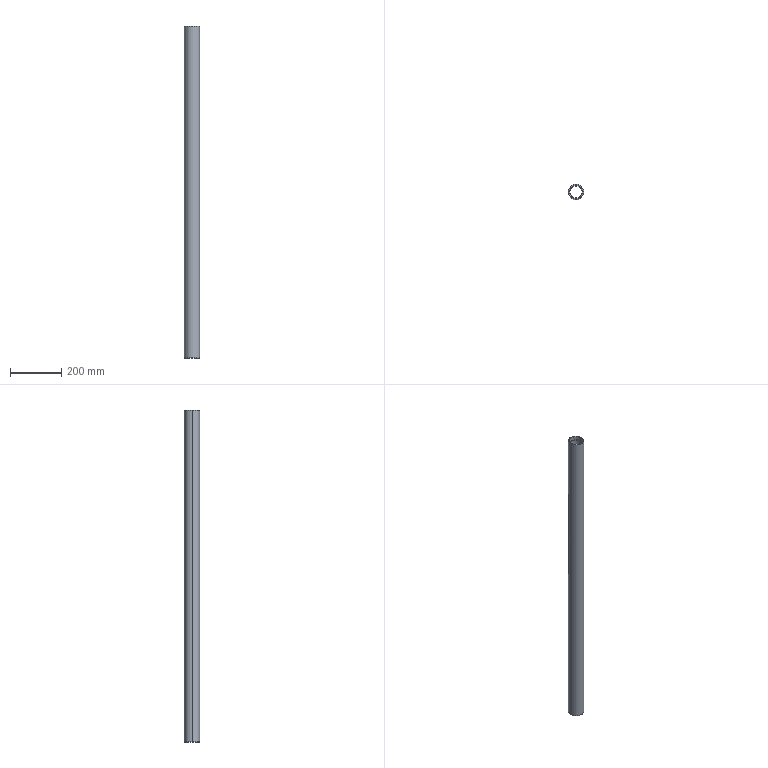Part | SolidWorks | features ICE 3, Chamfer 1, Extrusion 1 | 1 solid | 20 faces | box 60 x 60 x 1300 mm | volume 1313726 mm3 | cone 8 | cylinder 8 | plane 4 | commonest cylinder face diameters 52 x4 48 x2 60 x2
STEP:
#1=CARTESIAN_POINT('',(29.5,0.,1300.));
#2=VERTEX_POINT('',#1);
#3=CARTESIAN_POINT('',(-29.5,0.,1300.));
#4=VERTEX_POINT('',#3);
#5=CARTESIAN_POINT('',(0.,0.,1300.));
#6=DIRECTION('',(0.,0.,1.));
#7=DIRECTION('',(1.,0.,0.));
#8=AXIS2_PLACEMENT_3D('',#5,#6,#7);
#9=CIRCLE('',#8,29.5);
#10=EDGE_CURVE('',#2,#4,#9,.T.);
#11=ORIENTED_EDGE('',*,*,#10,.F.);
#12=CARTESIAN_POINT('',(30.,0.,1299.5));
#13=VERTEX_POINT('',#12);
#14=CARTESIAN_POINT('',(29.5,0.,1300.));
#15=DIRECTION('',(0.7071,0.,-0.7071));
#16=VECTOR('',#15,1000.);
#17=LINE('',#14,#16);
#18=EDGE_CURVE('',#2,#13,#17,.T.);
#19=ORIENTED_EDGE('',*,*,#18,.T.);
#20=CARTESIAN_POINT('',(-30.,0.,1299.5));
#21=VERTEX_POINT('',#20);
#22=CARTESIAN_POINT('',(0.,0.,1299.5));
#23=DIRECTION('',(0.,0.,-1.));
#24=DIRECTION('',(1.,0.,0.));
#25=AXIS2_PLACEMENT_3D('',#22,#23,#24);
#26=CIRCLE('',#25,30.);
#27=EDGE_CURVE('',#21,#13,#26,.T.);
#28=ORIENTED_EDGE('',*,*,#27,.F.);
#29=CARTESIAN_POINT('',(-29.5,0.,1300.));
#30=DIRECTION('',(-0.7071,0.,-0.7071));
#31=VECTOR('',#30,1000.);
#32=LINE('',#29,#31);
#33=EDGE_CURVE('',#4,#21,#32,.T.);
#34=ORIENTED_EDGE('',*,*,#33,.F.);
#35=EDGE_LOOP('',(#11,#19,#28,#34));
#36=FACE_OUTER_BOUND('',#35,.T.);
#37=CARTESIAN_POINT('',(0.,0.,1300.));
#38=DIRECTION('',(0.,0.,-1.));
#39=DIRECTION('',(-1.,0.,0.));
#40=AXIS2_PLACEMENT_3D('',#37,#38,#39);
#41=CONICAL_SURFACE('',#40,29.5,0.7854);
#42=ADVANCED_FACE('',(#36),#41,.T.);
#43=CARTESIAN_POINT('',(-26.,0.,1299.5));
#44=VERTEX_POINT('',#43);
#45=CARTESIAN_POINT('',(26.,0.,1299.5));
#46=VERTEX_POINT('',#45);
#47=CARTESIAN_POINT('',(0.,0.,1299.5));
#48=DIRECTION('',(0.,0.,1.));
#49=DIRECTION('',(1.,0.,0.));
#50=AXIS2_PLACEMENT_3D('',#47,#48,#49);
#51=CIRCLE('',#50,26.);
#52=EDGE_CURVE('',#44,#46,#51,.T.);
#53=ORIENTED_EDGE('',*,*,#52,.F.);
#54=CARTESIAN_POINT('',(-26.5,0.,1300.));
#55=VERTEX_POINT('',#54);
#56=CARTESIAN_POINT('',(-26.,0.,1299.5));
#57=DIRECTION('',(-0.7071,0.,0.7071));
#58=VECTOR('',#57,1000.);
#59=LINE('',#56,#58);
#60=EDGE_CURVE('',#44,#55,#59,.T.);
#61=ORIENTED_EDGE('',*,*,#60,.T.);
#62=CARTESIAN_POINT('',(26.5,0.,1300.));
#63=VERTEX_POINT('',#62);
#64=CARTESIAN_POINT('',(0.,0.,1300.));
#65=DIRECTION('',(0.,0.,-1.));
#66=DIRECTION('',(1.,0.,0.));
#67=AXIS2_PLACEMENT_3D('',#64,#65,#66);
#68=CIRCLE('',#67,26.5);
#69=EDGE_CURVE('',#63,#55,#68,.T.);
#70=ORIENTED_EDGE('',*,*,#69,.F.);
#71=CARTESIAN_POINT('',(26.,0.,1299.5));
#72=DIRECTION('',(0.7071,0.,0.7071));
#73=VECTOR('',#72,1000.);
#74=LINE('',#71,#73);
#75=EDGE_CURVE('',#46,#63,#74,.T.);
#76=ORIENTED_EDGE('',*,*,#75,.F.);
#77=EDGE_LOOP('',(#53,#61,#70,#76));
#78=FACE_OUTER_BOUND('',#77,.T.);
#79=CARTESIAN_POINT('',(0.,0.,1299.5));
#80=DIRECTION('',(0.,0.,1.));
#81=DIRECTION('',(1.,0.,0.));
#82=AXIS2_PLACEMENT_3D('',#79,#80,#81);
#83=CONICAL_SURFACE('',#82,26.,0.7854);
#84=ADVANCED_FACE('',(#78),#83,.F.);
#85=CARTESIAN_POINT('',(-29.5,0.,0.));
#86=VERTEX_POINT('',#85);
#87=CARTESIAN_POINT('',(29.5,0.,0.));
#88=VERTEX_POINT('',#87);
#89=CARTESIAN_POINT('',(0.,0.,0.));
#90=DIRECTION('',(0.,0.,-1.));
#91=DIRECTION('',(1.,0.,0.));
#92=AXIS2_PLACEMENT_3D('',#89,#90,#91);
#93=CIRCLE('',#92,29.5);
#94=EDGE_CURVE('',#86,#88,#93,.T.);
#95=ORIENTED_EDGE('',*,*,#94,.F.);
#96=CARTESIAN_POINT('',(-30.,0.,0.5));
#97=VERTEX_POINT('',#96);
#98=CARTESIAN_POINT('',(-30.,0.,0.5));
#99=DIRECTION('',(-0.7071,0.,0.7071));
#100=VECTOR('',#99,1000.);
#101=LINE('',#98,#100);
#102=EDGE_CURVE('',#86,#97,#101,.T.);
#103=ORIENTED_EDGE('',*,*,#102,.T.);
#104=CARTESIAN_POINT('',(30.,0.,0.5));
#105=VERTEX_POINT('',#104);
#106=CARTESIAN_POINT('',(0.,0.,0.5));
#107=DIRECTION('',(0.,0.,1.));
#108=DIRECTION('',(1.,0.,0.));
#109=AXIS2_PLACEMENT_3D('',#106,#107,#108);
#110=CIRCLE('',#109,30.);
#111=EDGE_CURVE('',#105,#97,#110,.T.);
#112=ORIENTED_EDGE('',*,*,#111,.F.);
#113=CARTESIAN_POINT('',(30.,0.,0.5));
#114=DIRECTION('',(0.7071,0.,0.7071));
#115=VECTOR('',#114,1000.);
#116=LINE('',#113,#115);
#117=EDGE_CURVE('',#88,#105,#116,.T.);
#118=ORIENTED_EDGE('',*,*,#117,.F.);
#119=EDGE_LOOP('',(#95,#103,#112,#118));
#120=FACE_OUTER_BOUND('',#119,.T.);
#121=CARTESIAN_POINT('',(0.,0.,0.5));
#122=DIRECTION('',(0.,0.,1.));
#123=DIRECTION('',(1.,0.,0.));
#124=AXIS2_PLACEMENT_3D('',#121,#122,#123);
#125=CONICAL_SURFACE('',#124,30.,0.7854);
#126=ADVANCED_FACE('',(#120),#125,.T.);
#127=CARTESIAN_POINT('',(26.,0.,0.5));
#128=VERTEX_POINT('',#127);
#129=CARTESIAN_POINT('',(-26.,0.,0.5));
#130=VERTEX_POINT('',#129);
#131=CARTESIAN_POINT('',(0.,0.,0.5));
#132=DIRECTION('',(0.,0.,-1.));
#133=DIRECTION('',(1.,0.,0.));
#134=AXIS2_PLACEMENT_3D('',#131,#132,#133);
#135=CIRCLE('',#134,26.);
#136=EDGE_CURVE('',#128,#130,#135,.T.);
#137=ORIENTED_EDGE('',*,*,#136,.F.);
#138=CARTESIAN_POINT('',(26.5,0.,0.));
#139=VERTEX_POINT('',#138);
#140=CARTESIAN_POINT('',(26.,0.,0.5));
#141=DIRECTION('',(0.7071,0.,-0.7071));
#142=VECTOR('',#141,1000.);
#143=LINE('',#140,#142);
#144=EDGE_CURVE('',#128,#139,#143,.T.);
#145=ORIENTED_EDGE('',*,*,#144,.T.);
#146=CARTESIAN_POINT('',(-26.5,0.,0.));
#147=VERTEX_POINT('',#146);
#148=CARTESIAN_POINT('',(0.,0.,0.));
#149=DIRECTION('',(0.,0.,1.));
#150=DIRECTION('',(1.,0.,0.));
#151=AXIS2_PLACEMENT_3D('',#148,#149,#150);
#152=CIRCLE('',#151,26.5);
#153=EDGE_CURVE('',#147,#139,#152,.T.);
#154=ORIENTED_EDGE('',*,*,#153,.F.);
#155=CARTESIAN_POINT('',(-26.,0.,0.5));
#156=DIRECTION('',(-0.7071,0.,-0.7071));
#157=VECTOR('',#156,1000.);
#158=LINE('',#155,#157);
#159=EDGE_CURVE('',#130,#147,#158,.T.);
#160=ORIENTED_EDGE('',*,*,#159,.F.);
#161=EDGE_LOOP('',(#137,#145,#154,#160));
#162=FACE_OUTER_BOUND('',#161,.T.);
#163=CARTESIAN_POINT('',(0.,0.,0.5));
#164=DIRECTION('',(0.,0.,-1.));
#165=DIRECTION('',(-1.,0.,0.));
#166=AXIS2_PLACEMENT_3D('',#163,#164,#165);
#167=CONICAL_SURFACE('',#166,26.,0.7854);
#168=ADVANCED_FACE('',(#162),#167,.F.);
#169=CARTESIAN_POINT('',(-26.,0.,1285.));
#170=VERTEX_POINT('',#169);
#171=CARTESIAN_POINT('',(26.,0.,1285.));
#172=VERTEX_POINT('',#171);
#173=CARTESIAN_POINT('',(0.,0.,1285.));
#174=DIRECTION('',(0.,0.,1.));
#175=DIRECTION('',(1.,0.,0.));
#176=AXIS2_PLACEMENT_3D('',#173,#174,#175);
#177=CIRCLE('',#176,26.);
#178=EDGE_CURVE('',#170,#172,#177,.T.);
#179=ORIENTED_EDGE('',*,*,#178,.F.);
#180=CARTESIAN_POINT('',(-26.,0.,1285.));
#181=DIRECTION('',(0.,0.,1.));
#182=VECTOR('',#181,1000.);
#183=LINE('',#180,#182);
#184=EDGE_CURVE('',#170,#44,#183,.T.);
#185=ORIENTED_EDGE('',*,*,#184,.T.);
#186=ORIENTED_EDGE('',*,*,#52,.T.);
#187=CARTESIAN_POINT('',(26.,0.,1285.));
#188=DIRECTION('',(0.,0.,1.));
#189=VECTOR('',#188,1000.);
#190=LINE('',#187,#189);
#191=EDGE_CURVE('',#172,#46,#190,.T.);
#192=ORIENTED_EDGE('',*,*,#191,.F.);
#193=EDGE_LOOP('',(#179,#185,#186,#192));
#194=FACE_OUTER_BOUND('',#193,.T.);
#195=CARTESIAN_POINT('',(0.,0.,1285.));
#196=DIRECTION('',(0.,0.,1.));
#197=DIRECTION('',(1.,0.,0.));
#198=AXIS2_PLACEMENT_3D('',#195,#196,#197);
#199=CYLINDRICAL_SURFACE('',#198,26.);
#200=ADVANCED_FACE('',(#194),#199,.F.);
#201=CARTESIAN_POINT('',(26.,0.,15.));
#202=VERTEX_POINT('',#201);
#203=CARTESIAN_POINT('',(-26.,0.,15.));
#204=VERTEX_POINT('',#203);
#205=CARTESIAN_POINT('',(0.,0.,15.));
#206=DIRECTION('',(0.,0.,-1.));
#207=DIRECTION('',(-1.,0.,0.));
#208=AXIS2_PLACEMENT_3D('',#205,#206,#207);
#209=CIRCLE('',#208,26.);
#210=EDGE_CURVE('',#202,#204,#209,.T.);
#211=ORIENTED_EDGE('',*,*,#210,.F.);
#212=CARTESIAN_POINT('',(26.,0.,15.));
#213=DIRECTION('',(0.,0.,-1.));
#214=VECTOR('',#213,1000.);
#215=LINE('',#212,#214);
#216=EDGE_CURVE('',#202,#128,#215,.T.);
#217=ORIENTED_EDGE('',*,*,#216,.T.);
#218=ORIENTED_EDGE('',*,*,#136,.T.);
#219=CARTESIAN_POINT('',(-26.,0.,15.));
#220=DIRECTION('',(0.,0.,-1.));
#221=VECTOR('',#220,1000.);
#222=LINE('',#219,#221);
#223=EDGE_CURVE('',#204,#130,#222,.T.);
#224=ORIENTED_EDGE('',*,*,#223,.F.);
#225=EDGE_LOOP('',(#211,#217,#218,#224));
#226=FACE_OUTER_BOUND('',#225,.T.);
#227=CARTESIAN_POINT('',(0.,0.,15.));
#228=DIRECTION('',(0.,0.,-1.));
#229=DIRECTION('',(-1.,0.,0.));
#230=AXIS2_PLACEMENT_3D('',#227,#228,#229);
#231=CYLINDRICAL_SURFACE('',#230,26.);
#232=ADVANCED_FACE('',(#226),#231,.F.);
#233=ORIENTED_EDGE('',*,*,#27,.T.);
#234=CARTESIAN_POINT('',(30.,0.,1300.));
#235=DIRECTION('',(0.,0.,-1.));
#236=VECTOR('',#235,1000.);
#237=LINE('',#234,#236);
#238=EDGE_CURVE('',#13,#105,#237,.T.);
#239=ORIENTED_EDGE('',*,*,#238,.T.);
#240=ORIENTED_EDGE('',*,*,#111,.T.);
#241=CARTESIAN_POINT('',(-30.,0.,1300.));
#242=DIRECTION('',(0.,0.,-1.));
#243=VECTOR('',#242,1000.);
#244=LINE('',#241,#243);
#245=EDGE_CURVE('',#21,#97,#244,.T.);
#246=ORIENTED_EDGE('',*,*,#245,.F.);
#247=EDGE_LOOP('',(#233,#239,#240,#246));
#248=FACE_OUTER_BOUND('',#247,.T.);
#249=CARTESIAN_POINT('',(0.,0.,1300.));
#250=DIRECTION('',(0.,0.,-1.));
#251=DIRECTION('',(-1.,0.,0.));
#252=AXIS2_PLACEMENT_3D('',#249,#250,#251);
#253=CYLINDRICAL_SURFACE('',#252,30.);
#254=ADVANCED_FACE('',(#248),#253,.T.);
#255=CARTESIAN_POINT('',(24.,0.,1285.));
#256=VERTEX_POINT('',#255);
#257=CARTESIAN_POINT('',(-24.,0.,1285.));
#258=VERTEX_POINT('',#257);
#259=CARTESIAN_POINT('',(0.,0.,1285.));
#260=DIRECTION('',(0.,0.,-1.));
#261=DIRECTION('',(1.,0.,0.));
#262=AXIS2_PLACEMENT_3D('',#259,#260,#261);
#263=CIRCLE('',#262,24.);
#264=EDGE_CURVE('',#256,#258,#263,.T.);
#265=ORIENTED_EDGE('',*,*,#264,.F.);
#266=CARTESIAN_POINT('',(24.,0.,15.));
#267=VERTEX_POINT('',#266);
#268=CARTESIAN_POINT('',(24.,0.,1600.));
#269=DIRECTION('',(0.,0.,-1.));
#270=VECTOR('',#269,1000.);
#271=LINE('',#268,#270);
#272=EDGE_CURVE('',#256,#267,#271,.T.);
#273=ORIENTED_EDGE('',*,*,#272,.T.);
#274=CARTESIAN_POINT('',(-24.,0.,15.));
#275=VERTEX_POINT('',#274);
#276=CARTESIAN_POINT('',(0.,0.,15.));
#277=DIRECTION('',(0.,0.,1.));
#278=DIRECTION('',(-1.,0.,0.));
#279=AXIS2_PLACEMENT_3D('',#276,#277,#278);
#280=CIRCLE('',#279,24.);
#281=EDGE_CURVE('',#275,#267,#280,.T.);
#282=ORIENTED_EDGE('',*,*,#281,.F.);
#283=CARTESIAN_POINT('',(-24.,0.,1600.));
#284=DIRECTION('',(0.,0.,-1.));
#285=VECTOR('',#284,1000.);
#286=LINE('',#283,#285);
#287=EDGE_CURVE('',#258,#275,#286,.T.);
#288=ORIENTED_EDGE('',*,*,#287,.F.);
#289=EDGE_LOOP('',(#265,#273,#282,#288));
#290=FACE_OUTER_BOUND('',#289,.T.);
#291=CARTESIAN_POINT('',(0.,0.,1600.));
#292=DIRECTION('',(0.,0.,-1.));
#293=DIRECTION('',(-1.,0.,0.));
#294=AXIS2_PLACEMENT_3D('',#291,#292,#293);
#295=CYLINDRICAL_SURFACE('',#294,24.);
#296=ADVANCED_FACE('',(#290),#295,.F.);
#297=ORIENTED_EDGE('',*,*,#272,.F.);
#298=CARTESIAN_POINT('',(0.,0.,1285.));
#299=DIRECTION('',(0.,0.,-1.));
#300=DIRECTION('',(1.,0.,0.));
#301=AXIS2_PLACEMENT_3D('',#298,#299,#300);
#302=CIRCLE('',#301,24.);
#303=EDGE_CURVE('',#258,#256,#302,.T.);
#304=ORIENTED_EDGE('',*,*,#303,.F.);
#305=ORIENTED_EDGE('',*,*,#287,.T.);
#306=CARTESIAN_POINT('',(0.,0.,15.));
#307=DIRECTION('',(0.,0.,1.));
#308=DIRECTION('',(-1.,0.,0.));
#309=AXIS2_PLACEMENT_3D('',#306,#307,#308);
#310=CIRCLE('',#309,24.);
#311=EDGE_CURVE('',#267,#275,#310,.T.);
#312=ORIENTED_EDGE('',*,*,#311,.F.);
#313=EDGE_LOOP('',(#297,#304,#305,#312));
#314=FACE_OUTER_BOUND('',#313,.T.);
#315=CARTESIAN_POINT('',(0.,0.,1600.));
#316=DIRECTION('',(0.,0.,-1.));
#317=DIRECTION('',(-1.,0.,0.));
#318=AXIS2_PLACEMENT_3D('',#315,#316,#317);
#319=CYLINDRICAL_SURFACE('',#318,24.);
#320=ADVANCED_FACE('',(#314),#319,.F.);
#321=ORIENTED_EDGE('',*,*,#238,.F.);
#322=CARTESIAN_POINT('',(0.,0.,1299.5));
#323=DIRECTION('',(0.,0.,-1.));
#324=DIRECTION('',(1.,0.,0.));
#325=AXIS2_PLACEMENT_3D('',#322,#323,#324);
#326=CIRCLE('',#325,30.);
#327=EDGE_CURVE('',#13,#21,#326,.T.);
#328=ORIENTED_EDGE('',*,*,#327,.T.);
#329=ORIENTED_EDGE('',*,*,#245,.T.);
#330=CARTESIAN_POINT('',(0.,0.,0.5));
#331=DIRECTION('',(0.,0.,1.));
#332=DIRECTION('',(1.,0.,0.));
#333=AXIS2_PLACEMENT_3D('',#330,#331,#332);
#334=CIRCLE('',#333,30.);
#335=EDGE_CURVE('',#97,#105,#334,.T.);
#336=ORIENTED_EDGE('',*,*,#335,.T.);
#337=EDGE_LOOP('',(#321,#328,#329,#336));
#338=FACE_OUTER_BOUND('',#337,.T.);
#339=CARTESIAN_POINT('',(0.,0.,1300.));
#340=DIRECTION('',(0.,0.,-1.));
#341=DIRECTION('',(-1.,0.,0.));
#342=AXIS2_PLACEMENT_3D('',#339,#340,#341);
#343=CYLINDRICAL_SURFACE('',#342,30.);
#344=ADVANCED_FACE('',(#338),#343,.T.);
#345=ORIENTED_EDGE('',*,*,#69,.T.);
#346=CARTESIAN_POINT('',(0.,0.,1300.));
#347=DIRECTION('',(0.,0.,-1.));
#348=DIRECTION('',(1.,0.,0.));
#349=AXIS2_PLACEMENT_3D('',#346,#347,#348);
#350=CIRCLE('',#349,26.5);
#351=EDGE_CURVE('',#55,#63,#350,.T.);
#352=ORIENTED_EDGE('',*,*,#351,.T.);
#353=EDGE_LOOP('',(#345,#352));
#354=FACE_BOUND('',#353,.T.);
#355=CARTESIAN_POINT('',(0.,0.,1300.));
#356=DIRECTION('',(0.,0.,1.));
#357=DIRECTION('',(1.,0.,0.));
#358=AXIS2_PLACEMENT_3D('',#355,#356,#357);
#359=CIRCLE('',#358,29.5);
#360=EDGE_CURVE('',#4,#2,#359,.T.);
#361=ORIENTED_EDGE('',*,*,#360,.T.);
#362=ORIENTED_EDGE('',*,*,#10,.T.);
#363=EDGE_LOOP('',(#361,#362));
#364=FACE_OUTER_BOUND('',#363,.T.);
#365=CARTESIAN_POINT('',(0.,0.,1300.));
#366=DIRECTION('',(0.,0.,1.));
#367=DIRECTION('',(1.,0.,0.));
#368=AXIS2_PLACEMENT_3D('',#365,#366,#367);
#369=PLANE('',#368);
#370=ADVANCED_FACE('',(#354,#364),#369,.T.);
#371=ORIENTED_EDGE('',*,*,#153,.T.);
#372=CARTESIAN_POINT('',(0.,0.,0.));
#373=DIRECTION('',(0.,0.,1.));
#374=DIRECTION('',(1.,0.,0.));
#375=AXIS2_PLACEMENT_3D('',#372,#373,#374);
#376=CIRCLE('',#375,26.5);
#377=EDGE_CURVE('',#139,#147,#376,.T.);
#378=ORIENTED_EDGE('',*,*,#377,.T.);
#379=EDGE_LOOP('',(#371,#378));
#380=FACE_BOUND('',#379,.T.);
#381=CARTESIAN_POINT('',(0.,0.,0.));
#382=DIRECTION('',(0.,0.,-1.));
#383=DIRECTION('',(1.,0.,0.));
#384=AXIS2_PLACEMENT_3D('',#381,#382,#383);
#385=CIRCLE('',#384,29.5);
#386=EDGE_CURVE('',#88,#86,#385,.T.);
#387=ORIENTED_EDGE('',*,*,#386,.T.);
#388=ORIENTED_EDGE('',*,*,#94,.T.);
#389=EDGE_LOOP('',(#387,#388));
#390=FACE_OUTER_BOUND('',#389,.T.);
#391=CARTESIAN_POINT('',(0.,0.,0.));
#392=DIRECTION('',(0.,0.,1.));
#393=DIRECTION('',(1.,0.,0.));
#394=AXIS2_PLACEMENT_3D('',#391,#392,#393);
#395=PLANE('',#394);
#396=ADVANCED_FACE('',(#380,#390),#395,.F.);
#397=CARTESIAN_POINT('',(0.,0.,15.));
#398=DIRECTION('',(0.,0.,-1.));
#399=DIRECTION('',(-1.,0.,0.));
#400=AXIS2_PLACEMENT_3D('',#397,#398,#399);
#401=CIRCLE('',#400,26.);
#402=EDGE_CURVE('',#204,#202,#401,.T.);
#403=ORIENTED_EDGE('',*,*,#402,.T.);
#404=ORIENTED_EDGE('',*,*,#210,.T.);
#405=EDGE_LOOP('',(#403,#404));
#406=FACE_OUTER_BOUND('',#405,.T.);
#407=ORIENTED_EDGE('',*,*,#281,.T.);
#408=ORIENTED_EDGE('',*,*,#311,.T.);
#409=EDGE_LOOP('',(#407,#408));
#410=FACE_BOUND('',#409,.T.);
#411=CARTESIAN_POINT('',(0.,0.,15.));
#412=DIRECTION('',(0.,0.,-1.));
#413=DIRECTION('',(-1.,0.,0.));
#414=AXIS2_PLACEMENT_3D('',#411,#412,#413);
#415=PLANE('',#414);
#416=ADVANCED_FACE('',(#406,#410),#415,.T.);
#417=ORIENTED_EDGE('',*,*,#216,.F.);
#418=ORIENTED_EDGE('',*,*,#402,.F.);
#419=ORIENTED_EDGE('',*,*,#223,.T.);
#420=CARTESIAN_POINT('',(0.,0.,0.5));
#421=DIRECTION('',(0.,0.,-1.));
#422=DIRECTION('',(1.,0.,0.));
#423=AXIS2_PLACEMENT_3D('',#420,#421,#422);
#424=CIRCLE('',#423,26.);
#425=EDGE_CURVE('',#130,#128,#424,.T.);
#426=ORIENTED_EDGE('',*,*,#425,.T.);
#427=EDGE_LOOP('',(#417,#418,#419,#426));
#428=FACE_OUTER_BOUND('',#427,.T.);
#429=CARTESIAN_POINT('',(0.,0.,15.));
#430=DIRECTION('',(0.,0.,-1.));
#431=DIRECTION('',(-1.,0.,0.));
#432=AXIS2_PLACEMENT_3D('',#429,#430,#431);
#433=CYLINDRICAL_SURFACE('',#432,26.);
#434=ADVANCED_FACE('',(#428),#433,.F.);
#435=CARTESIAN_POINT('',(0.,0.,1285.));
#436=DIRECTION('',(0.,0.,1.));
#437=DIRECTION('',(1.,0.,0.));
#438=AXIS2_PLACEMENT_3D('',#435,#436,#437);
#439=CIRCLE('',#438,26.);
#440=EDGE_CURVE('',#172,#170,#439,.T.);
#441=ORIENTED_EDGE('',*,*,#440,.T.);
#442=ORIENTED_EDGE('',*,*,#178,.T.);
#443=EDGE_LOOP('',(#441,#442));
#444=FACE_OUTER_BOUND('',#443,.T.);
#445=ORIENTED_EDGE('',*,*,#303,.T.);
#446=ORIENTED_EDGE('',*,*,#264,.T.);
#447=EDGE_LOOP('',(#445,#446));
#448=FACE_BOUND('',#447,.T.);
#449=CARTESIAN_POINT('',(0.,0.,1285.));
#450=DIRECTION('',(0.,0.,1.));
#451=DIRECTION('',(1.,0.,0.));
#452=AXIS2_PLACEMENT_3D('',#449,#450,#451);
#453=PLANE('',#452);
#454=ADVANCED_FACE('',(#444,#448),#453,.T.);
#455=ORIENTED_EDGE('',*,*,#184,.F.);
#456=ORIENTED_EDGE('',*,*,#440,.F.);
#457=ORIENTED_EDGE('',*,*,#191,.T.);
#458=CARTESIAN_POINT('',(0.,0.,1299.5));
#459=DIRECTION('',(0.,0.,1.));
#460=DIRECTION('',(1.,0.,0.));
#461=AXIS2_PLACEMENT_3D('',#458,#459,#460);
#462=CIRCLE('',#461,26.);
#463=EDGE_CURVE('',#46,#44,#462,.T.);
#464=ORIENTED_EDGE('',*,*,#463,.T.);
#465=EDGE_LOOP('',(#455,#456,#457,#464));
#466=FACE_OUTER_BOUND('',#465,.T.);
#467=CARTESIAN_POINT('',(0.,0.,1285.));
#468=DIRECTION('',(0.,0.,1.));
#469=DIRECTION('',(1.,0.,0.));
#470=AXIS2_PLACEMENT_3D('',#467,#468,#469);
#471=CYLINDRICAL_SURFACE('',#470,26.);
#472=ADVANCED_FACE('',(#466),#471,.F.);
#473=ORIENTED_EDGE('',*,*,#144,.F.);
#474=ORIENTED_EDGE('',*,*,#425,.F.);
#475=ORIENTED_EDGE('',*,*,#159,.T.);
#476=ORIENTED_EDGE('',*,*,#377,.F.);
#477=EDGE_LOOP('',(#473,#474,#475,#476));
#478=FACE_OUTER_BOUND('',#477,.T.);
#479=CARTESIAN_POINT('',(0.,0.,0.5));
#480=DIRECTION('',(0.,0.,-1.));
#481=DIRECTION('',(-1.,0.,0.));
#482=AXIS2_PLACEMENT_3D('',#479,#480,#481);
#483=CONICAL_SURFACE('',#482,26.,0.7854);
#484=ADVANCED_FACE('',(#478),#483,.F.);
#485=ORIENTED_EDGE('',*,*,#102,.F.);
#486=ORIENTED_EDGE('',*,*,#386,.F.);
#487=ORIENTED_EDGE('',*,*,#117,.T.);
#488=ORIENTED_EDGE('',*,*,#335,.F.);
#489=EDGE_LOOP('',(#485,#486,#487,#488));
#490=FACE_OUTER_BOUND('',#489,.T.);
#491=CARTESIAN_POINT('',(0.,0.,0.5));
#492=DIRECTION('',(0.,0.,1.));
#493=DIRECTION('',(1.,0.,0.));
#494=AXIS2_PLACEMENT_3D('',#491,#492,#493);
#495=CONICAL_SURFACE('',#494,30.,0.7854);
#496=ADVANCED_FACE('',(#490),#495,.T.);
#497=ORIENTED_EDGE('',*,*,#60,.F.);
#498=ORIENTED_EDGE('',*,*,#463,.F.);
#499=ORIENTED_EDGE('',*,*,#75,.T.);
#500=ORIENTED_EDGE('',*,*,#351,.F.);
#501=EDGE_LOOP('',(#497,#498,#499,#500));
#502=FACE_OUTER_BOUND('',#501,.T.);
#503=CARTESIAN_POINT('',(0.,0.,1299.5));
#504=DIRECTION('',(0.,0.,1.));
#505=DIRECTION('',(1.,0.,0.));
#506=AXIS2_PLACEMENT_3D('',#503,#504,#505);
#507=CONICAL_SURFACE('',#506,26.,0.7854);
#508=ADVANCED_FACE('',(#502),#507,.F.);
#509=ORIENTED_EDGE('',*,*,#18,.F.);
#510=ORIENTED_EDGE('',*,*,#360,.F.);
#511=ORIENTED_EDGE('',*,*,#33,.T.);
#512=ORIENTED_EDGE('',*,*,#327,.F.);
#513=EDGE_LOOP('',(#509,#510,#511,#512));
#514=FACE_OUTER_BOUND('',#513,.T.);
#515=CARTESIAN_POINT('',(0.,0.,1300.));
#516=DIRECTION('',(0.,0.,-1.));
#517=DIRECTION('',(-1.,0.,0.));
#518=AXIS2_PLACEMENT_3D('',#515,#516,#517);
#519=CONICAL_SURFACE('',#518,29.5,0.7854);
#520=ADVANCED_FACE('',(#514),#519,.T.);
#521=CLOSED_SHELL('',(#42,#84,#126,#168,#200,#232,#254,#296,#320,#344,#370,#396,#416,#434,#454,#472,#484,#496,#508,#520));
#522=MANIFOLD_SOLID_BREP('',#521);
#523=CARTESIAN_POINT('',(0.,0.,0.));
#524=DIRECTION('',(0.,0.,1.));
#525=DIRECTION('',(1.,0.,0.));
#526=AXIS2_PLACEMENT_3D('',#523,#524,#525);
#527=(LENGTH_UNIT()NAMED_UNIT(*)SI_UNIT(.MILLI.,.METRE.));
#528=UNCERTAINTY_MEASURE_WITH_UNIT(LENGTH_MEASURE(0.00001),#527,'','');
#529=(NAMED_UNIT(*)PLANE_ANGLE_UNIT()SI_UNIT($,.RADIAN.));
#530=(NAMED_UNIT(*)SI_UNIT($,.STERADIAN.)SOLID_ANGLE_UNIT());
#531=(GEOMETRIC_REPRESENTATION_CONTEXT(3)GLOBAL_UNCERTAINTY_ASSIGNED_CONTEXT((#528))GLOBAL_UNIT_ASSIGNED_CONTEXT((#527,#529,#530))REPRESENTATION_CONTEXT('',''));
#532=ADVANCED_BREP_SHAPE_REPRESENTATION('',(#522,#526),#531);